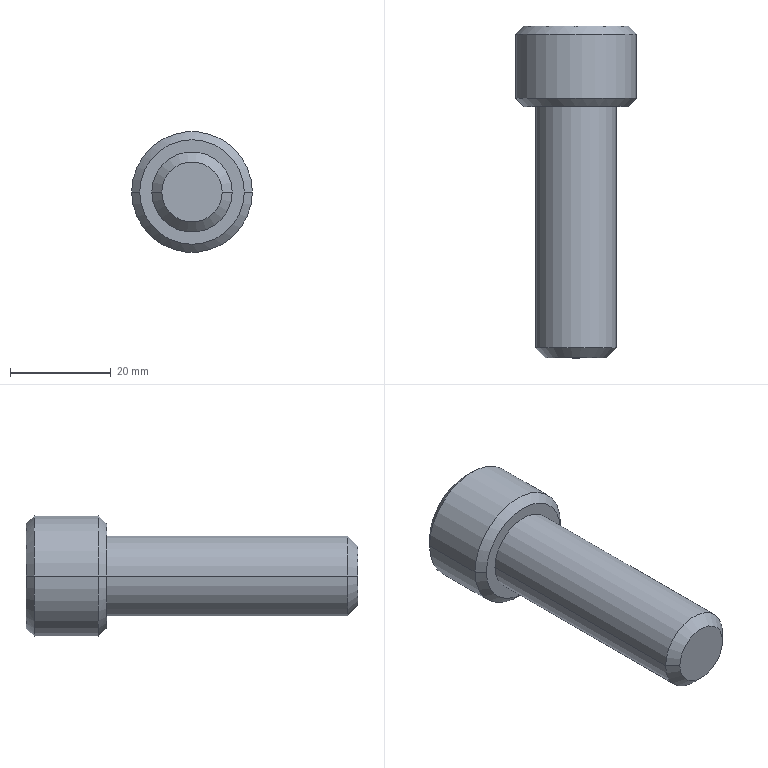Part | STEP file | BB62-M16-50L | 1 solid | 27 faces | box 24 x 66 x 24 mm | volume 15375 mm3 | plane 15 | cone 8 | cylinder 4 | commonest cylinder face diameters 16 x2 24 x2